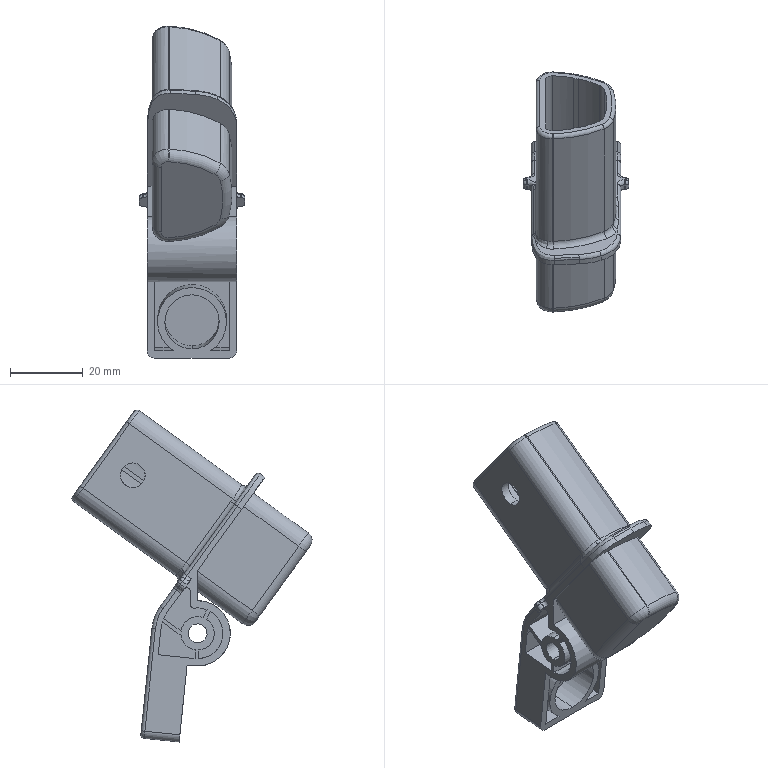Part | SolidWorks | features BaseBody 1 | 1 solid | 221 faces | box 29.203 x 66.154 x 91.497 mm | volume 22564 mm3 | cylinder 96 | plane 76 | torus 32 | spline 13 | sphere 4 | commonest cylinder face diameters 2 x32 9.2 x7 14 x7 9 x6 4 x5 20 x5